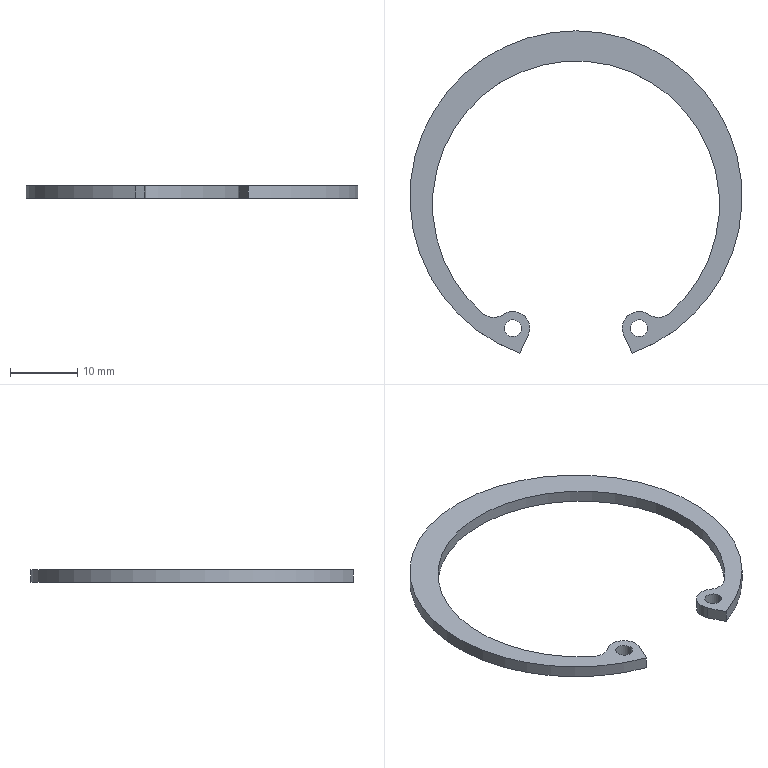Part | STEP file | KS B 1336 - 47x1.8 | 1 solid | 16 faces | box 49.5 x 48.026 x 1.8 mm | volume 847.052 mm3 | cylinder 12 | plane 4 | commonest cylinder face diameters 2.5 x4 5 x4 42.75 x2 49.5 x2
STEP:
#1=CARTESIAN_POINT('',(0.,0.,0.));
#2=DIRECTION('',(0.,0.,1.));
#3=DIRECTION('',(1.,0.,0.));
#4=AXIS2_PLACEMENT_3D('',#1,#2,#3);
#5=CARTESIAN_POINT('',(8.152,-43.058,0.));
#6=VERTEX_POINT('',#5);
#7=CARTESIAN_POINT('',(8.152,-43.058,1.8));
#8=VERTEX_POINT('',#7);
#9=CARTESIAN_POINT('',(8.152,-43.058,0.));
#10=DIRECTION('',(0.,0.,1.));
#11=VECTOR('',#10,1.);
#12=LINE('',#9,#11);
#13=CARTESIAN_POINT('',(9.402,-43.058,0.));
#14=DIRECTION('',(0.,0.,1.));
#15=DIRECTION('',(-1.,0.,0.));
#16=AXIS2_PLACEMENT_3D('',#13,#14,#15);
#17=CYLINDRICAL_SURFACE('',#16,1.25);
#18=CARTESIAN_POINT('',(6.283,0.));
#19=DIRECTION('',(0.,1.));
#20=VECTOR('',#19,1.);
#21=LINE('',#18,#20);
#22=(GEOMETRIC_REPRESENTATION_CONTEXT(2)PARAMETRIC_REPRESENTATION_CONTEXT()REPRESENTATION_CONTEXT('',''));
#23=DEFINITIONAL_REPRESENTATION('',(#21),#22);
#24=PCURVE('',#17,#23);
#25=CARTESIAN_POINT('',(9.402,-43.058,0.));
#26=DIRECTION('',(0.,0.,1.));
#27=DIRECTION('',(-1.,0.,0.));
#28=AXIS2_PLACEMENT_3D('',#25,#26,#27);
#29=CYLINDRICAL_SURFACE('',#28,1.25);
#30=CARTESIAN_POINT('',(0.,0.));
#31=DIRECTION('',(0.,1.));
#32=VECTOR('',#31,1.);
#33=LINE('',#30,#32);
#34=(GEOMETRIC_REPRESENTATION_CONTEXT(2)PARAMETRIC_REPRESENTATION_CONTEXT()REPRESENTATION_CONTEXT('',''));
#35=DEFINITIONAL_REPRESENTATION('',(#33),#34);
#36=PCURVE('',#29,#35);
#37=SURFACE_CURVE('',#12,(#24,#36),.PCURVE_S1.);
#38=EDGE_CURVE('',#6,#8,#37,.T.);
#39=ORIENTED_EDGE('',*,*,#38,.T.);
#40=CARTESIAN_POINT('',(10.652,-43.058,1.8));
#41=VERTEX_POINT('',#40);
#42=CARTESIAN_POINT('',(9.402,-43.058,1.8));
#43=DIRECTION('',(0.,0.,-1.));
#44=DIRECTION('',(-1.,0.,0.));
#45=AXIS2_PLACEMENT_3D('',#42,#43,#44);
#46=CIRCLE('',#45,1.25);
#47=CARTESIAN_POINT('',(6.283,1.8));
#48=DIRECTION('',(-1.,0.));
#49=VECTOR('',#48,1.);
#50=LINE('',#47,#49);
#51=(GEOMETRIC_REPRESENTATION_CONTEXT(2)PARAMETRIC_REPRESENTATION_CONTEXT()REPRESENTATION_CONTEXT('',''));
#52=DEFINITIONAL_REPRESENTATION('',(#50),#51);
#53=PCURVE('',#17,#52);
#54=CARTESIAN_POINT('',(-0.06336,-23.349,1.8));
#55=DIRECTION('',(0.,0.,1.));
#56=DIRECTION('',(1.,0.,0.));
#57=AXIS2_PLACEMENT_3D('',#54,#55,#56);
#58=PLANE('',#57);
#59=CARTESIAN_POINT('',(8.215,-19.708));
#60=CARTESIAN_POINT('',(8.215,-17.543));
#61=CARTESIAN_POINT('',(10.09,-18.626));
#62=CARTESIAN_POINT('',(11.965,-19.708));
#63=CARTESIAN_POINT('',(10.09,-20.791));
#64=CARTESIAN_POINT('',(8.215,-21.873));
#65=CARTESIAN_POINT('',(8.215,-19.708));
#66=(BOUNDED_CURVE()B_SPLINE_CURVE(2,(#59,#60,#61,#62,#63,#64,#65),.UNSPECIFIED.,.T.,.F.)B_SPLINE_CURVE_WITH_KNOTS((1,2,2,2,2,1),(-2.094,0.,2.094,4.189,6.283,8.378),.UNSPECIFIED.)CURVE()GEOMETRIC_REPRESENTATION_ITEM()RATIONAL_B_SPLINE_CURVE((1.,0.5,1.,0.5,1.,0.5,1.))REPRESENTATION_ITEM(''));
#67=(GEOMETRIC_REPRESENTATION_CONTEXT(2)PARAMETRIC_REPRESENTATION_CONTEXT()REPRESENTATION_CONTEXT('',''));
#68=DEFINITIONAL_REPRESENTATION('',(#66),#67);
#69=PCURVE('',#58,#68);
#70=SURFACE_CURVE('',#46,(#53,#69),.PCURVE_S1.);
#71=EDGE_CURVE('',#8,#41,#70,.T.);
#72=ORIENTED_EDGE('',*,*,#71,.T.);
#73=CARTESIAN_POINT('',(10.652,-43.058,0.));
#74=VERTEX_POINT('',#73);
#75=CARTESIAN_POINT('',(10.652,-43.058,0.));
#76=DIRECTION('',(0.,0.,1.));
#77=VECTOR('',#76,1.);
#78=LINE('',#75,#77);
#79=CARTESIAN_POINT('',(3.142,0.));
#80=DIRECTION('',(0.,1.));
#81=VECTOR('',#80,1.);
#82=LINE('',#79,#81);
#83=(GEOMETRIC_REPRESENTATION_CONTEXT(2)PARAMETRIC_REPRESENTATION_CONTEXT()REPRESENTATION_CONTEXT('',''));
#84=DEFINITIONAL_REPRESENTATION('',(#82),#83);
#85=PCURVE('',#17,#84);
#86=CARTESIAN_POINT('',(3.142,0.));
#87=DIRECTION('',(0.,1.));
#88=VECTOR('',#87,1.);
#89=LINE('',#86,#88);
#90=(GEOMETRIC_REPRESENTATION_CONTEXT(2)PARAMETRIC_REPRESENTATION_CONTEXT()REPRESENTATION_CONTEXT('',''));
#91=DEFINITIONAL_REPRESENTATION('',(#89),#90);
#92=PCURVE('',#29,#91);
#93=SURFACE_CURVE('',#78,(#85,#92),.PCURVE_S1.);
#94=EDGE_CURVE('',#74,#41,#93,.T.);
#95=ORIENTED_EDGE('',*,*,#94,.F.);
#96=CARTESIAN_POINT('',(9.402,-43.058,0.));
#97=DIRECTION('',(0.,0.,1.));
#98=DIRECTION('',(-1.,0.,0.));
#99=AXIS2_PLACEMENT_3D('',#96,#97,#98);
#100=CIRCLE('',#99,1.25);
#101=CARTESIAN_POINT('',(0.,0.));
#102=DIRECTION('',(1.,0.));
#103=VECTOR('',#102,1.);
#104=LINE('',#101,#103);
#105=(GEOMETRIC_REPRESENTATION_CONTEXT(2)PARAMETRIC_REPRESENTATION_CONTEXT()REPRESENTATION_CONTEXT('',''));
#106=DEFINITIONAL_REPRESENTATION('',(#104),#105);
#107=PCURVE('',#17,#106);
#108=CARTESIAN_POINT('',(-0.06336,-23.349,0.));
#109=DIRECTION('',(0.,0.,1.));
#110=DIRECTION('',(1.,0.,0.));
#111=AXIS2_PLACEMENT_3D('',#108,#109,#110);
#112=PLANE('',#111);
#113=CARTESIAN_POINT('',(9.465,-19.708));
#114=DIRECTION('',(-1.,0.));
#115=AXIS2_PLACEMENT_2D('',#113,#114);
#116=CIRCLE('',#115,1.25);
#117=(GEOMETRIC_REPRESENTATION_CONTEXT(2)PARAMETRIC_REPRESENTATION_CONTEXT()REPRESENTATION_CONTEXT('',''));
#118=DEFINITIONAL_REPRESENTATION('',(#116),#117);
#119=PCURVE('',#112,#118);
#120=SURFACE_CURVE('',#100,(#107,#119),.PCURVE_S1.);
#121=EDGE_CURVE('',#74,#6,#120,.T.);
#122=ORIENTED_EDGE('',*,*,#121,.T.);
#123=EDGE_LOOP('',(#39,#72,#95,#122));
#124=FACE_BOUND('',#123,.F.);
#125=ADVANCED_FACE('',(#124),#17,.F.);
#126=CARTESIAN_POINT('',(-10.652,-43.058,0.));
#127=VERTEX_POINT('',#126);
#128=CARTESIAN_POINT('',(-10.652,-43.058,1.8));
#129=VERTEX_POINT('',#128);
#130=CARTESIAN_POINT('',(-10.652,-43.058,0.));
#131=DIRECTION('',(0.,0.,1.));
#132=VECTOR('',#131,1.);
#133=LINE('',#130,#132);
#134=CARTESIAN_POINT('',(-9.402,-43.058,0.));
#135=DIRECTION('',(0.,0.,1.));
#136=DIRECTION('',(-1.,0.,0.));
#137=AXIS2_PLACEMENT_3D('',#134,#135,#136);
#138=CYLINDRICAL_SURFACE('',#137,1.25);
#139=CARTESIAN_POINT('',(6.283,0.));
#140=DIRECTION('',(0.,1.));
#141=VECTOR('',#140,1.);
#142=LINE('',#139,#141);
#143=(GEOMETRIC_REPRESENTATION_CONTEXT(2)PARAMETRIC_REPRESENTATION_CONTEXT()REPRESENTATION_CONTEXT('',''));
#144=DEFINITIONAL_REPRESENTATION('',(#142),#143);
#145=PCURVE('',#138,#144);
#146=CARTESIAN_POINT('',(-9.402,-43.058,0.));
#147=DIRECTION('',(0.,0.,1.));
#148=DIRECTION('',(-1.,0.,0.));
#149=AXIS2_PLACEMENT_3D('',#146,#147,#148);
#150=CYLINDRICAL_SURFACE('',#149,1.25);
#151=CARTESIAN_POINT('',(0.,0.));
#152=DIRECTION('',(0.,1.));
#153=VECTOR('',#152,1.);
#154=LINE('',#151,#153);
#155=(GEOMETRIC_REPRESENTATION_CONTEXT(2)PARAMETRIC_REPRESENTATION_CONTEXT()REPRESENTATION_CONTEXT('',''));
#156=DEFINITIONAL_REPRESENTATION('',(#154),#155);
#157=PCURVE('',#150,#156);
#158=SURFACE_CURVE('',#133,(#145,#157),.PCURVE_S1.);
#159=EDGE_CURVE('',#127,#129,#158,.T.);
#160=ORIENTED_EDGE('',*,*,#159,.T.);
#161=CARTESIAN_POINT('',(-8.152,-43.058,1.8));
#162=VERTEX_POINT('',#161);
#163=CARTESIAN_POINT('',(-9.402,-43.058,1.8));
#164=DIRECTION('',(0.,0.,-1.));
#165=DIRECTION('',(-1.,0.,0.));
#166=AXIS2_PLACEMENT_3D('',#163,#164,#165);
#167=CIRCLE('',#166,1.25);
#168=CARTESIAN_POINT('',(6.283,1.8));
#169=DIRECTION('',(-1.,0.));
#170=VECTOR('',#169,1.);
#171=LINE('',#168,#170);
#172=(GEOMETRIC_REPRESENTATION_CONTEXT(2)PARAMETRIC_REPRESENTATION_CONTEXT()REPRESENTATION_CONTEXT('',''));
#173=DEFINITIONAL_REPRESENTATION('',(#171),#172);
#174=PCURVE('',#138,#173);
#175=CARTESIAN_POINT('',(-10.588,-19.708));
#176=CARTESIAN_POINT('',(-10.588,-17.543));
#177=CARTESIAN_POINT('',(-8.713,-18.626));
#178=CARTESIAN_POINT('',(-6.838,-19.708));
#179=CARTESIAN_POINT('',(-8.713,-20.791));
#180=CARTESIAN_POINT('',(-10.588,-21.873));
#181=CARTESIAN_POINT('',(-10.588,-19.708));
#182=(BOUNDED_CURVE()B_SPLINE_CURVE(2,(#175,#176,#177,#178,#179,#180,#181),.UNSPECIFIED.,.T.,.F.)B_SPLINE_CURVE_WITH_KNOTS((1,2,2,2,2,1),(-2.094,0.,2.094,4.189,6.283,8.378),.UNSPECIFIED.)CURVE()GEOMETRIC_REPRESENTATION_ITEM()RATIONAL_B_SPLINE_CURVE((1.,0.5,1.,0.5,1.,0.5,1.))REPRESENTATION_ITEM(''));
#183=(GEOMETRIC_REPRESENTATION_CONTEXT(2)PARAMETRIC_REPRESENTATION_CONTEXT()REPRESENTATION_CONTEXT('',''));
#184=DEFINITIONAL_REPRESENTATION('',(#182),#183);
#185=PCURVE('',#58,#184);
#186=SURFACE_CURVE('',#167,(#174,#185),.PCURVE_S1.);
#187=EDGE_CURVE('',#129,#162,#186,.T.);
#188=ORIENTED_EDGE('',*,*,#187,.T.);
#189=CARTESIAN_POINT('',(-8.152,-43.058,0.));
#190=VERTEX_POINT('',#189);
#191=CARTESIAN_POINT('',(-8.152,-43.058,0.));
#192=DIRECTION('',(0.,0.,1.));
#193=VECTOR('',#192,1.);
#194=LINE('',#191,#193);
#195=CARTESIAN_POINT('',(3.142,0.));
#196=DIRECTION('',(0.,1.));
#197=VECTOR('',#196,1.);
#198=LINE('',#195,#197);
#199=(GEOMETRIC_REPRESENTATION_CONTEXT(2)PARAMETRIC_REPRESENTATION_CONTEXT()REPRESENTATION_CONTEXT('',''));
#200=DEFINITIONAL_REPRESENTATION('',(#198),#199);
#201=PCURVE('',#138,#200);
#202=CARTESIAN_POINT('',(3.142,0.));
#203=DIRECTION('',(0.,1.));
#204=VECTOR('',#203,1.);
#205=LINE('',#202,#204);
#206=(GEOMETRIC_REPRESENTATION_CONTEXT(2)PARAMETRIC_REPRESENTATION_CONTEXT()REPRESENTATION_CONTEXT('',''));
#207=DEFINITIONAL_REPRESENTATION('',(#205),#206);
#208=PCURVE('',#150,#207);
#209=SURFACE_CURVE('',#194,(#201,#208),.PCURVE_S1.);
#210=EDGE_CURVE('',#190,#162,#209,.T.);
#211=ORIENTED_EDGE('',*,*,#210,.F.);
#212=CARTESIAN_POINT('',(-9.402,-43.058,0.));
#213=DIRECTION('',(0.,0.,1.));
#214=DIRECTION('',(-1.,0.,0.));
#215=AXIS2_PLACEMENT_3D('',#212,#213,#214);
#216=CIRCLE('',#215,1.25);
#217=CARTESIAN_POINT('',(0.,0.));
#218=DIRECTION('',(1.,0.));
#219=VECTOR('',#218,1.);
#220=LINE('',#217,#219);
#221=(GEOMETRIC_REPRESENTATION_CONTEXT(2)PARAMETRIC_REPRESENTATION_CONTEXT()REPRESENTATION_CONTEXT('',''));
#222=DEFINITIONAL_REPRESENTATION('',(#220),#221);
#223=PCURVE('',#138,#222);
#224=CARTESIAN_POINT('',(-9.338,-19.708));
#225=DIRECTION('',(-1.,0.));
#226=AXIS2_PLACEMENT_2D('',#224,#225);
#227=CIRCLE('',#226,1.25);
#228=(GEOMETRIC_REPRESENTATION_CONTEXT(2)PARAMETRIC_REPRESENTATION_CONTEXT()REPRESENTATION_CONTEXT('',''));
#229=DEFINITIONAL_REPRESENTATION('',(#227),#228);
#230=PCURVE('',#112,#229);
#231=SURFACE_CURVE('',#216,(#223,#230),.PCURVE_S1.);
#232=EDGE_CURVE('',#190,#127,#231,.T.);
#233=ORIENTED_EDGE('',*,*,#232,.T.);
#234=EDGE_LOOP('',(#160,#188,#211,#233));
#235=FACE_BOUND('',#234,.F.);
#236=ADVANCED_FACE('',(#235),#138,.F.);
#237=CARTESIAN_POINT('',(-13.899,-40.864,0.));
#238=VERTEX_POINT('',#237);
#239=CARTESIAN_POINT('',(-13.899,-40.864,1.8));
#240=VERTEX_POINT('',#239);
#241=CARTESIAN_POINT('',(-13.899,-40.864,0.));
#242=DIRECTION('',(0.,0.,1.));
#243=VECTOR('',#242,1.);
#244=LINE('',#241,#243);
#245=CARTESIAN_POINT('',(0.,-24.625,0.));
#246=DIRECTION('',(0.,0.,1.));
#247=DIRECTION('',(-0.6503,0.7597,0.));
#248=AXIS2_PLACEMENT_3D('',#245,#246,#247);
#249=CYLINDRICAL_SURFACE('',#248,21.375);
#250=CARTESIAN_POINT('',(1.726,0.));
#251=DIRECTION('',(0.,1.));
#252=VECTOR('',#251,1.);
#253=LINE('',#250,#252);
#254=(GEOMETRIC_REPRESENTATION_CONTEXT(2)PARAMETRIC_REPRESENTATION_CONTEXT()REPRESENTATION_CONTEXT('',''));
#255=DEFINITIONAL_REPRESENTATION('',(#253),#254);
#256=PCURVE('',#249,#255);
#257=CARTESIAN_POINT('',(-12.274,-38.965,0.));
#258=DIRECTION('',(0.,0.,1.));
#259=DIRECTION('',(0.6503,0.7597,0.));
#260=AXIS2_PLACEMENT_3D('',#257,#258,#259);
#261=CYLINDRICAL_SURFACE('',#260,2.5);
#262=CARTESIAN_POINT('',(3.142,0.));
#263=DIRECTION('',(0.,1.));
#264=VECTOR('',#263,1.);
#265=LINE('',#262,#264);
#266=(GEOMETRIC_REPRESENTATION_CONTEXT(2)PARAMETRIC_REPRESENTATION_CONTEXT()REPRESENTATION_CONTEXT('',''));
#267=DEFINITIONAL_REPRESENTATION('',(#265),#266);
#268=PCURVE('',#261,#267);
#269=SURFACE_CURVE('',#244,(#256,#268),.PCURVE_S1.);
#270=EDGE_CURVE('',#238,#240,#269,.T.);
#271=ORIENTED_EDGE('',*,*,#270,.T.);
#272=CARTESIAN_POINT('',(-13.899,-8.386,1.8));
#273=VERTEX_POINT('',#272);
#274=CARTESIAN_POINT('',(0.,-24.625,1.8));
#275=DIRECTION('',(0.,0.,1.));
#276=DIRECTION('',(-0.6503,0.7597,0.));
#277=AXIS2_PLACEMENT_3D('',#274,#275,#276);
#278=CIRCLE('',#277,21.375);
#279=CARTESIAN_POINT('',(0.,1.8));
#280=DIRECTION('',(1.,0.));
#281=VECTOR('',#280,1.);
#282=LINE('',#279,#281);
#283=(GEOMETRIC_REPRESENTATION_CONTEXT(2)PARAMETRIC_REPRESENTATION_CONTEXT()REPRESENTATION_CONTEXT('',''));
#284=DEFINITIONAL_REPRESENTATION('',(#282),#283);
#285=PCURVE('',#249,#284);
#286=CARTESIAN_POINT('',(0.06336,-1.276));
#287=DIRECTION('',(-0.6503,0.7597));
#288=AXIS2_PLACEMENT_2D('',#286,#287);
#289=CIRCLE('',#288,21.375);
#290=(GEOMETRIC_REPRESENTATION_CONTEXT(2)PARAMETRIC_REPRESENTATION_CONTEXT()REPRESENTATION_CONTEXT('',''));
#291=DEFINITIONAL_REPRESENTATION('',(#289),#290);
#292=PCURVE('',#58,#291);
#293=SURFACE_CURVE('',#278,(#285,#292),.PCURVE_S1.);
#294=EDGE_CURVE('',#273,#240,#293,.T.);
#295=ORIENTED_EDGE('',*,*,#294,.F.);
#296=CARTESIAN_POINT('',(-13.899,-8.386,0.));
#297=VERTEX_POINT('',#296);
#298=CARTESIAN_POINT('',(-13.899,-8.386,0.));
#299=DIRECTION('',(0.,0.,1.));
#300=VECTOR('',#299,1.);
#301=LINE('',#298,#300);
#302=CARTESIAN_POINT('',(0.,0.));
#303=DIRECTION('',(0.,1.));
#304=VECTOR('',#303,1.);
#305=LINE('',#302,#304);
#306=(GEOMETRIC_REPRESENTATION_CONTEXT(2)PARAMETRIC_REPRESENTATION_CONTEXT()REPRESENTATION_CONTEXT('',''));
#307=DEFINITIONAL_REPRESENTATION('',(#305),#306);
#308=PCURVE('',#249,#307);
#309=CARTESIAN_POINT('',(0.,-24.625,0.));
#310=DIRECTION('',(0.,0.,1.));
#311=DIRECTION('',(-0.6503,0.7597,0.));
#312=AXIS2_PLACEMENT_3D('',#309,#310,#311);
#313=CYLINDRICAL_SURFACE('',#312,21.375);
#314=CARTESIAN_POINT('',(6.283,0.));
#315=DIRECTION('',(0.,1.));
#316=VECTOR('',#315,1.);
#317=LINE('',#314,#316);
#318=(GEOMETRIC_REPRESENTATION_CONTEXT(2)PARAMETRIC_REPRESENTATION_CONTEXT()REPRESENTATION_CONTEXT('',''));
#319=DEFINITIONAL_REPRESENTATION('',(#317),#318);
#320=PCURVE('',#313,#319);
#321=SURFACE_CURVE('',#301,(#308,#320),.PCURVE_S1.);
#322=EDGE_CURVE('',#297,#273,#321,.T.);
#323=ORIENTED_EDGE('',*,*,#322,.F.);
#324=CARTESIAN_POINT('',(0.,-24.625,0.));
#325=DIRECTION('',(0.,0.,-1.));
#326=DIRECTION('',(-0.6503,0.7597,0.));
#327=AXIS2_PLACEMENT_3D('',#324,#325,#326);
#328=CIRCLE('',#327,21.375);
#329=CARTESIAN_POINT('',(6.283,0.));
#330=DIRECTION('',(-1.,0.));
#331=VECTOR('',#330,1.);
#332=LINE('',#329,#331);
#333=(GEOMETRIC_REPRESENTATION_CONTEXT(2)PARAMETRIC_REPRESENTATION_CONTEXT()REPRESENTATION_CONTEXT('',''));
#334=DEFINITIONAL_REPRESENTATION('',(#332),#333);
#335=PCURVE('',#249,#334);
#336=CARTESIAN_POINT('',(-13.836,14.963));
#337=CARTESIAN_POINT('',(14.291,39.037));
#338=CARTESIAN_POINT('',(21.076,2.642));
#339=CARTESIAN_POINT('',(27.862,-33.754));
#340=CARTESIAN_POINT('',(-7.05,-21.432));
#341=CARTESIAN_POINT('',(-41.963,-9.111));
#342=CARTESIAN_POINT('',(-13.836,14.963));
#343=(BOUNDED_CURVE()B_SPLINE_CURVE(2,(#336,#337,#338,#339,#340,#341,#342),.UNSPECIFIED.,.T.,.F.)B_SPLINE_CURVE_WITH_KNOTS((1,2,2,2,2,1),(-2.094,0.,2.094,4.189,6.283,8.378),.UNSPECIFIED.)CURVE()GEOMETRIC_REPRESENTATION_ITEM()RATIONAL_B_SPLINE_CURVE((1.,0.5,1.,0.5,1.,0.5,1.))REPRESENTATION_ITEM(''));
#344=(GEOMETRIC_REPRESENTATION_CONTEXT(2)PARAMETRIC_REPRESENTATION_CONTEXT()REPRESENTATION_CONTEXT('',''));
#345=DEFINITIONAL_REPRESENTATION('',(#343),#344);
#346=PCURVE('',#112,#345);
#347=SURFACE_CURVE('',#328,(#335,#346),.PCURVE_S1.);
#348=EDGE_CURVE('',#238,#297,#347,.T.);
#349=ORIENTED_EDGE('',*,*,#348,.F.);
#350=EDGE_LOOP('',(#271,#295,#323,#349));
#351=FACE_BOUND('',#350,.F.);
#352=ADVANCED_FACE('',(#351),#249,.F.);
#353=CARTESIAN_POINT('',(8.415,-46.776,0.));
#354=VERTEX_POINT('',#353);
#355=CARTESIAN_POINT('',(0.,1.25,0.));
#356=VERTEX_POINT('',#355);
#357=CARTESIAN_POINT('',(0.,-23.5,0.));
#358=DIRECTION('',(0.,0.,1.));
#359=DIRECTION('',(0.34,-0.9404,0.));
#360=AXIS2_PLACEMENT_3D('',#357,#358,#359);
#361=CIRCLE('',#360,24.75);
#362=CARTESIAN_POINT('',(0.,-23.5,0.));
#363=DIRECTION('',(0.,0.,1.));
#364=DIRECTION('',(0.,1.,0.));
#365=AXIS2_PLACEMENT_3D('',#362,#363,#364);
#366=CYLINDRICAL_SURFACE('',#365,24.75);
#367=CARTESIAN_POINT('',(3.489,0.));
#368=DIRECTION('',(1.,0.));
#369=VECTOR('',#368,1.);
#370=LINE('',#367,#369);
#371=(GEOMETRIC_REPRESENTATION_CONTEXT(2)PARAMETRIC_REPRESENTATION_CONTEXT()REPRESENTATION_CONTEXT('',''));
#372=DEFINITIONAL_REPRESENTATION('',(#370),#371);
#373=PCURVE('',#366,#372);
#374=CARTESIAN_POINT('',(0.06336,-0.1508));
#375=DIRECTION('',(0.34,-0.9404));
#376=AXIS2_PLACEMENT_2D('',#374,#375);
#377=CIRCLE('',#376,24.75);
#378=(GEOMETRIC_REPRESENTATION_CONTEXT(2)PARAMETRIC_REPRESENTATION_CONTEXT()REPRESENTATION_CONTEXT('',''));
#379=DEFINITIONAL_REPRESENTATION('',(#377),#378);
#380=PCURVE('',#112,#379);
#381=SURFACE_CURVE('',#361,(#373,#380),.PCURVE_S1.);
#382=EDGE_CURVE('',#354,#356,#381,.T.);
#383=ORIENTED_EDGE('',*,*,#382,.T.);
#384=CARTESIAN_POINT('',(0.,1.25,1.8));
#385=VERTEX_POINT('',#384);
#386=CARTESIAN_POINT('',(0.,1.25,0.));
#387=DIRECTION('',(0.,0.,1.));
#388=VECTOR('',#387,1.);
#389=LINE('',#386,#388);
#390=CARTESIAN_POINT('',(6.283,0.));
#391=DIRECTION('',(0.,1.));
#392=VECTOR('',#391,1.);
#393=LINE('',#390,#392);
#394=(GEOMETRIC_REPRESENTATION_CONTEXT(2)PARAMETRIC_REPRESENTATION_CONTEXT()REPRESENTATION_CONTEXT('',''));
#395=DEFINITIONAL_REPRESENTATION('',(#393),#394);
#396=PCURVE('',#366,#395);
#397=CARTESIAN_POINT('',(0.,-23.5,0.));
#398=DIRECTION('',(0.,0.,1.));
#399=DIRECTION('',(0.,1.,0.));
#400=AXIS2_PLACEMENT_3D('',#397,#398,#399);
#401=CYLINDRICAL_SURFACE('',#400,24.75);
#402=CARTESIAN_POINT('',(0.,0.));
#403=DIRECTION('',(0.,1.));
#404=VECTOR('',#403,1.);
#405=LINE('',#402,#404);
#406=(GEOMETRIC_REPRESENTATION_CONTEXT(2)PARAMETRIC_REPRESENTATION_CONTEXT()REPRESENTATION_CONTEXT('',''));
#407=DEFINITIONAL_REPRESENTATION('',(#405),#406);
#408=PCURVE('',#401,#407);
#409=SURFACE_CURVE('',#389,(#396,#408),.PCURVE_S1.);
#410=EDGE_CURVE('',#356,#385,#409,.T.);
#411=ORIENTED_EDGE('',*,*,#410,.T.);
#412=CARTESIAN_POINT('',(8.415,-46.776,1.8));
#413=VERTEX_POINT('',#412);
#414=CARTESIAN_POINT('',(0.,-23.5,1.8));
#415=DIRECTION('',(0.,0.,-1.));
#416=DIRECTION('',(0.34,-0.9404,0.));
#417=AXIS2_PLACEMENT_3D('',#414,#415,#416);
#418=CIRCLE('',#417,24.75);
#419=CARTESIAN_POINT('',(9.772,1.8));
#420=DIRECTION('',(-1.,0.));
#421=VECTOR('',#420,1.);
#422=LINE('',#419,#421);
#423=(GEOMETRIC_REPRESENTATION_CONTEXT(2)PARAMETRIC_REPRESENTATION_CONTEXT()REPRESENTATION_CONTEXT('',''));
#424=DEFINITIONAL_REPRESENTATION('',(#422),#423);
#425=PCURVE('',#366,#424);
#426=CARTESIAN_POINT('',(8.478,-23.426));
#427=CARTESIAN_POINT('',(-31.836,-38.002));
#428=CARTESIAN_POINT('',(-24.301,4.199));
#429=CARTESIAN_POINT('',(-16.767,46.4));
#430=CARTESIAN_POINT('',(16.013,18.775));
#431=CARTESIAN_POINT('',(48.793,-8.851));
#432=CARTESIAN_POINT('',(8.478,-23.426));
#433=(BOUNDED_CURVE()B_SPLINE_CURVE(2,(#426,#427,#428,#429,#430,#431,#432),.UNSPECIFIED.,.T.,.F.)B_SPLINE_CURVE_WITH_KNOTS((1,2,2,2,2,1),(-2.094,0.,2.094,4.189,6.283,8.378),.UNSPECIFIED.)CURVE()GEOMETRIC_REPRESENTATION_ITEM()RATIONAL_B_SPLINE_CURVE((1.,0.5,1.,0.5,1.,0.5,1.))REPRESENTATION_ITEM(''));
#434=(GEOMETRIC_REPRESENTATION_CONTEXT(2)PARAMETRIC_REPRESENTATION_CONTEXT()REPRESENTATION_CONTEXT('',''));
#435=DEFINITIONAL_REPRESENTATION('',(#433),#434);
#436=PCURVE('',#58,#435);
#437=SURFACE_CURVE('',#418,(#425,#436),.PCURVE_S1.);
#438=EDGE_CURVE('',#385,#413,#437,.T.);
#439=ORIENTED_EDGE('',*,*,#438,.T.);
#440=CARTESIAN_POINT('',(8.415,-46.776,0.));
#441=DIRECTION('',(0.,0.,1.));
#442=VECTOR('',#441,1.);
#443=LINE('',#440,#442);
#444=CARTESIAN_POINT('',(3.489,0.));
#445=DIRECTION('',(0.,1.));
#446=VECTOR('',#445,1.);
#447=LINE('',#444,#446);
#448=(GEOMETRIC_REPRESENTATION_CONTEXT(2)PARAMETRIC_REPRESENTATION_CONTEXT()REPRESENTATION_CONTEXT('',''));
#449=DEFINITIONAL_REPRESENTATION('',(#447),#448);
#450=PCURVE('',#366,#449);
#451=CARTESIAN_POINT('',(8.415,-46.776,0.));
#452=DIRECTION('',(-0.9013,-0.4333,0.));
#453=DIRECTION('',(-0.4333,0.9013,0.));
#454=AXIS2_PLACEMENT_3D('',#451,#452,#453);
#455=PLANE('',#454);
#456=CARTESIAN_POINT('',(0.,0.));
#457=DIRECTION('',(0.,-1.));
#458=VECTOR('',#457,1.);
#459=LINE('',#456,#458);
#460=(GEOMETRIC_REPRESENTATION_CONTEXT(2)PARAMETRIC_REPRESENTATION_CONTEXT()REPRESENTATION_CONTEXT('',''));
#461=DEFINITIONAL_REPRESENTATION('',(#459),#460);
#462=PCURVE('',#455,#461);
#463=SURFACE_CURVE('',#443,(#450,#462),.PCURVE_S1.);
#464=EDGE_CURVE('',#354,#413,#463,.T.);
#465=ORIENTED_EDGE('',*,*,#464,.F.);
#466=EDGE_LOOP('',(#383,#411,#439,#465));
#467=FACE_BOUND('',#466,.T.);
#468=ADVANCED_FACE('',(#467),#366,.T.);
#469=ORIENTED_EDGE('',*,*,#187,.T.);
#470=CARTESIAN_POINT('',(-9.402,-43.058,1.8));
#471=DIRECTION('',(0.,0.,-1.));
#472=DIRECTION('',(-1.,0.,0.));
#473=AXIS2_PLACEMENT_3D('',#470,#471,#472);
#474=CIRCLE('',#473,1.25);
#475=CARTESIAN_POINT('',(-10.588,-19.708));
#476=CARTESIAN_POINT('',(-10.588,-17.543));
#477=CARTESIAN_POINT('',(-8.713,-18.626));
#478=CARTESIAN_POINT('',(-6.838,-19.708));
#479=CARTESIAN_POINT('',(-8.713,-20.791));
#480=CARTESIAN_POINT('',(-10.588,-21.873));
#481=CARTESIAN_POINT('',(-10.588,-19.708));
#482=(BOUNDED_CURVE()B_SPLINE_CURVE(2,(#475,#476,#477,#478,#479,#480,#481),.UNSPECIFIED.,.T.,.F.)B_SPLINE_CURVE_WITH_KNOTS((1,2,2,2,2,1),(-2.094,0.,2.094,4.189,6.283,8.378),.UNSPECIFIED.)CURVE()GEOMETRIC_REPRESENTATION_ITEM()RATIONAL_B_SPLINE_CURVE((1.,0.5,1.,0.5,1.,0.5,1.))REPRESENTATION_ITEM(''));
#483=(GEOMETRIC_REPRESENTATION_CONTEXT(2)PARAMETRIC_REPRESENTATION_CONTEXT()REPRESENTATION_CONTEXT('',''));
#484=DEFINITIONAL_REPRESENTATION('',(#482),#483);
#485=PCURVE('',#58,#484);
#486=CARTESIAN_POINT('',(6.283,1.8));
#487=DIRECTION('',(-1.,0.));
#488=VECTOR('',#487,1.);
#489=LINE('',#486,#488);
#490=(GEOMETRIC_REPRESENTATION_CONTEXT(2)PARAMETRIC_REPRESENTATION_CONTEXT()REPRESENTATION_CONTEXT('',''));
#491=DEFINITIONAL_REPRESENTATION('',(#489),#490);
#492=PCURVE('',#150,#491);
#493=SURFACE_CURVE('',#474,(#485,#492),.PCURVE_S1.);
#494=EDGE_CURVE('',#162,#129,#493,.T.);
#495=ORIENTED_EDGE('',*,*,#494,.T.);
#496=EDGE_LOOP('',(#469,#495));
#497=FACE_BOUND('',#496,.T.);
#498=ORIENTED_EDGE('',*,*,#71,.T.);
#499=CARTESIAN_POINT('',(9.402,-43.058,1.8));
#500=DIRECTION('',(0.,0.,-1.));
#501=DIRECTION('',(-1.,0.,0.));
#502=AXIS2_PLACEMENT_3D('',#499,#500,#501);
#503=CIRCLE('',#502,1.25);
#504=CARTESIAN_POINT('',(8.215,-19.708));
#505=CARTESIAN_POINT('',(8.215,-17.543));
#506=CARTESIAN_POINT('',(10.09,-18.626));
#507=CARTESIAN_POINT('',(11.965,-19.708));
#508=CARTESIAN_POINT('',(10.09,-20.791));
#509=CARTESIAN_POINT('',(8.215,-21.873));
#510=CARTESIAN_POINT('',(8.215,-19.708));
#511=(BOUNDED_CURVE()B_SPLINE_CURVE(2,(#504,#505,#506,#507,#508,#509,#510),.UNSPECIFIED.,.T.,.F.)B_SPLINE_CURVE_WITH_KNOTS((1,2,2,2,2,1),(-2.094,0.,2.094,4.189,6.283,8.378),.UNSPECIFIED.)CURVE()GEOMETRIC_REPRESENTATION_ITEM()RATIONAL_B_SPLINE_CURVE((1.,0.5,1.,0.5,1.,0.5,1.))REPRESENTATION_ITEM(''));
#512=(GEOMETRIC_REPRESENTATION_CONTEXT(2)PARAMETRIC_REPRESENTATION_CONTEXT()REPRESENTATION_CONTEXT('',''));
#513=DEFINITIONAL_REPRESENTATION('',(#511),#512);
#514=PCURVE('',#58,#513);
#515=CARTESIAN_POINT('',(6.283,1.8));
#516=DIRECTION('',(-1.,0.));
#517=VECTOR('',#516,1.);
#518=LINE('',#515,#517);
#519=(GEOMETRIC_REPRESENTATION_CONTEXT(2)PARAMETRIC_REPRESENTATION_CONTEXT()REPRESENTATION_CONTEXT('',''));
#520=DEFINITIONAL_REPRESENTATION('',(#518),#519);
#521=PCURVE('',#29,#520);
#522=SURFACE_CURVE('',#503,(#514,#521),.PCURVE_S1.);
#523=EDGE_CURVE('',#41,#8,#522,.T.);
#524=ORIENTED_EDGE('',*,*,#523,.T.);
#525=EDGE_LOOP('',(#498,#524));
#526=FACE_BOUND('',#525,.T.);
#527=CARTESIAN_POINT('',(13.899,-40.864,1.8));
#528=VERTEX_POINT('',#527);
#529=CARTESIAN_POINT('',(0.,-24.625,1.8));
#530=DIRECTION('',(0.,0.,1.));
#531=DIRECTION('',(-0.6503,0.7597,0.));
#532=AXIS2_PLACEMENT_3D('',#529,#530,#531);
#533=CIRCLE('',#532,21.375);
#534=CARTESIAN_POINT('',(0.06336,-1.276));
#535=DIRECTION('',(-0.6503,0.7597));
#536=AXIS2_PLACEMENT_2D('',#534,#535);
#537=CIRCLE('',#536,21.375);
#538=(GEOMETRIC_REPRESENTATION_CONTEXT(2)PARAMETRIC_REPRESENTATION_CONTEXT()REPRESENTATION_CONTEXT('',''));
#539=DEFINITIONAL_REPRESENTATION('',(#537),#538);
#540=PCURVE('',#58,#539);
#541=CARTESIAN_POINT('',(0.,1.8));
#542=DIRECTION('',(1.,0.));
#543=VECTOR('',#542,1.);
#544=LINE('',#541,#543);
#545=(GEOMETRIC_REPRESENTATION_CONTEXT(2)PARAMETRIC_REPRESENTATION_CONTEXT()REPRESENTATION_CONTEXT('',''));
#546=DEFINITIONAL_REPRESENTATION('',(#544),#545);
#547=PCURVE('',#313,#546);
#548=SURFACE_CURVE('',#533,(#540,#547),.PCURVE_S1.);
#549=EDGE_CURVE('',#528,#273,#548,.T.);
#550=ORIENTED_EDGE('',*,*,#549,.F.);
#551=CARTESIAN_POINT('',(10.838,-41.011,1.8));
#552=VERTEX_POINT('',#551);
#553=CARTESIAN_POINT('',(12.274,-38.965,1.8));
#554=DIRECTION('',(0.,0.,1.));
#555=DIRECTION('',(0.5744,0.8186,0.));
#556=AXIS2_PLACEMENT_3D('',#553,#554,#555);
#557=CIRCLE('',#556,2.5);
#558=CARTESIAN_POINT('',(12.337,-15.615));
#559=DIRECTION('',(0.5744,0.8186));
#560=AXIS2_PLACEMENT_2D('',#558,#559);
#561=CIRCLE('',#560,2.5);
#562=(GEOMETRIC_REPRESENTATION_CONTEXT(2)PARAMETRIC_REPRESENTATION_CONTEXT()REPRESENTATION_CONTEXT('',''));
#563=DEFINITIONAL_REPRESENTATION('',(#561),#562);
#564=PCURVE('',#58,#563);
#565=CARTESIAN_POINT('',(12.274,-38.965,0.));
#566=DIRECTION('',(0.,0.,1.));
#567=DIRECTION('',(0.5744,0.8186,0.));
#568=AXIS2_PLACEMENT_3D('',#565,#566,#567);
#569=CYLINDRICAL_SURFACE('',#568,2.5);
#570=CARTESIAN_POINT('',(0.,1.8));
#571=DIRECTION('',(1.,0.));
#572=VECTOR('',#571,1.);
#573=LINE('',#570,#572);
#574=(GEOMETRIC_REPRESENTATION_CONTEXT(2)PARAMETRIC_REPRESENTATION_CONTEXT()REPRESENTATION_CONTEXT('',''));
#575=DEFINITIONAL_REPRESENTATION('',(#573),#574);
#576=PCURVE('',#569,#575);
#577=SURFACE_CURVE('',#557,(#564,#576),.PCURVE_S1.);
#578=EDGE_CURVE('',#552,#528,#577,.T.);
#579=ORIENTED_EDGE('',*,*,#578,.F.);
#580=CARTESIAN_POINT('',(7.148,-44.141,1.8));
#581=VERTEX_POINT('',#580);
#582=CARTESIAN_POINT('',(9.402,-43.058,1.8));
#583=DIRECTION('',(0.,0.,-1.));
#584=DIRECTION('',(0.5744,0.8186,0.));
#585=AXIS2_PLACEMENT_3D('',#582,#583,#584);
#586=CIRCLE('',#585,2.5);
#587=CARTESIAN_POINT('',(10.901,-17.662));
#588=CARTESIAN_POINT('',(14.446,-20.149));
#589=CARTESIAN_POINT('',(10.519,-21.975));
#590=CARTESIAN_POINT('',(6.593,-23.801));
#591=CARTESIAN_POINT('',(6.975,-19.488));
#592=CARTESIAN_POINT('',(7.356,-15.175));
#593=CARTESIAN_POINT('',(10.901,-17.662));
#594=(BOUNDED_CURVE()B_SPLINE_CURVE(2,(#587,#588,#589,#590,#591,#592,#593),.UNSPECIFIED.,.T.,.F.)B_SPLINE_CURVE_WITH_KNOTS((1,2,2,2,2,1),(-2.094,0.,2.094,4.189,6.283,8.378),.UNSPECIFIED.)CURVE()GEOMETRIC_REPRESENTATION_ITEM()RATIONAL_B_SPLINE_CURVE((1.,0.5,1.,0.5,1.,0.5,1.))REPRESENTATION_ITEM(''));
#595=(GEOMETRIC_REPRESENTATION_CONTEXT(2)PARAMETRIC_REPRESENTATION_CONTEXT()REPRESENTATION_CONTEXT('',''));
#596=DEFINITIONAL_REPRESENTATION('',(#594),#595);
#597=PCURVE('',#58,#596);
#598=CARTESIAN_POINT('',(9.402,-43.058,0.));
#599=DIRECTION('',(0.,0.,1.));
#600=DIRECTION('',(0.5744,0.8186,0.));
#601=AXIS2_PLACEMENT_3D('',#598,#599,#600);
#602=CYLINDRICAL_SURFACE('',#601,2.5);
#603=CARTESIAN_POINT('',(6.283,1.8));
#604=DIRECTION('',(-1.,0.));
#605=VECTOR('',#604,1.);
#606=LINE('',#603,#605);
#607=(GEOMETRIC_REPRESENTATION_CONTEXT(2)PARAMETRIC_REPRESENTATION_CONTEXT()REPRESENTATION_CONTEXT('',''));
#608=DEFINITIONAL_REPRESENTATION('',(#606),#607);
#609=PCURVE('',#602,#608);
#610=SURFACE_CURVE('',#586,(#597,#609),.PCURVE_S1.);
#611=EDGE_CURVE('',#581,#552,#610,.T.);
#612=ORIENTED_EDGE('',*,*,#611,.F.);
#613=CARTESIAN_POINT('',(7.148,-44.141,1.8));
#614=DIRECTION('',(-0.4333,0.9013,0.));
#615=VECTOR('',#614,1.);
#616=LINE('',#613,#615);
#617=CARTESIAN_POINT('',(7.212,-20.792));
#618=DIRECTION('',(-0.4333,0.9013));
#619=VECTOR('',#618,1.);
#620=LINE('',#617,#619);
#621=(GEOMETRIC_REPRESENTATION_CONTEXT(2)PARAMETRIC_REPRESENTATION_CONTEXT()REPRESENTATION_CONTEXT('',''));
#622=DEFINITIONAL_REPRESENTATION('',(#620),#621);
#623=PCURVE('',#58,#622);
#624=CARTESIAN_POINT('',(2.923,-1.8));
#625=DIRECTION('',(1.,0.));
#626=VECTOR('',#625,1.);
#627=LINE('',#624,#626);
#628=(GEOMETRIC_REPRESENTATION_CONTEXT(2)PARAMETRIC_REPRESENTATION_CONTEXT()REPRESENTATION_CONTEXT('',''));
#629=DEFINITIONAL_REPRESENTATION('',(#627),#628);
#630=PCURVE('',#455,#629);
#631=SURFACE_CURVE('',#616,(#623,#630),.PCURVE_S1.);
#632=EDGE_CURVE('',#413,#581,#631,.T.);
#633=ORIENTED_EDGE('',*,*,#632,.F.);
#634=ORIENTED_EDGE('',*,*,#438,.F.);
#635=CARTESIAN_POINT('',(-8.415,-46.776,1.8));
#636=VERTEX_POINT('',#635);
#637=CARTESIAN_POINT('',(0.,-23.5,1.8));
#638=DIRECTION('',(0.,0.,-1.));
#639=DIRECTION('',(0.34,-0.9404,0.));
#640=AXIS2_PLACEMENT_3D('',#637,#638,#639);
#641=CIRCLE('',#640,24.75);
#642=CARTESIAN_POINT('',(8.478,-23.426));
#643=CARTESIAN_POINT('',(-31.836,-38.002));
#644=CARTESIAN_POINT('',(-24.301,4.199));
#645=CARTESIAN_POINT('',(-16.767,46.4));
#646=CARTESIAN_POINT('',(16.013,18.775));
#647=CARTESIAN_POINT('',(48.793,-8.851));
#648=CARTESIAN_POINT('',(8.478,-23.426));
#649=(BOUNDED_CURVE()B_SPLINE_CURVE(2,(#642,#643,#644,#645,#646,#647,#648),.UNSPECIFIED.,.T.,.F.)B_SPLINE_CURVE_WITH_KNOTS((1,2,2,2,2,1),(-2.094,0.,2.094,4.189,6.283,8.378),.UNSPECIFIED.)CURVE()GEOMETRIC_REPRESENTATION_ITEM()RATIONAL_B_SPLINE_CURVE((1.,0.5,1.,0.5,1.,0.5,1.))REPRESENTATION_ITEM(''));
#650=(GEOMETRIC_REPRESENTATION_CONTEXT(2)PARAMETRIC_REPRESENTATION_CONTEXT()REPRESENTATION_CONTEXT('',''));
#651=DEFINITIONAL_REPRESENTATION('',(#649),#650);
#652=PCURVE('',#58,#651);
#653=CARTESIAN_POINT('',(3.489,1.8));
#654=DIRECTION('',(-1.,0.));
#655=VECTOR('',#654,1.);
#656=LINE('',#653,#655);
#657=(GEOMETRIC_REPRESENTATION_CONTEXT(2)PARAMETRIC_REPRESENTATION_CONTEXT()REPRESENTATION_CONTEXT('',''));
#658=DEFINITIONAL_REPRESENTATION('',(#656),#657);
#659=PCURVE('',#401,#658);
#660=SURFACE_CURVE('',#641,(#652,#659),.PCURVE_S1.);
#661=EDGE_CURVE('',#636,#385,#660,.T.);
#662=ORIENTED_EDGE('',*,*,#661,.F.);
#663=CARTESIAN_POINT('',(-7.148,-44.141,1.8));
#664=VERTEX_POINT('',#663);
#665=CARTESIAN_POINT('',(-8.415,-46.776,1.8));
#666=DIRECTION('',(-0.4333,-0.9013,0.));
#667=VECTOR('',#666,1.);
#668=LINE('',#665,#667);
#669=CARTESIAN_POINT('',(-8.352,-23.426));
#670=DIRECTION('',(-0.4333,-0.9013));
#671=VECTOR('',#670,1.);
#672=LINE('',#669,#671);
#673=(GEOMETRIC_REPRESENTATION_CONTEXT(2)PARAMETRIC_REPRESENTATION_CONTEXT()REPRESENTATION_CONTEXT('',''));
#674=DEFINITIONAL_REPRESENTATION('',(#672),#673);
#675=PCURVE('',#58,#674);
#676=CARTESIAN_POINT('',(-7.148,-44.141,0.));
#677=DIRECTION('',(0.9013,-0.4333,0.));
#678=DIRECTION('',(0.,0.,-1.));
#679=AXIS2_PLACEMENT_3D('',#676,#677,#678);
#680=PLANE('',#679);
#681=CARTESIAN_POINT('',(-1.8,-2.923));
#682=DIRECTION('',(0.,-1.));
#683=VECTOR('',#682,1.);
#684=LINE('',#681,#683);
#685=(GEOMETRIC_REPRESENTATION_CONTEXT(2)PARAMETRIC_REPRESENTATION_CONTEXT()REPRESENTATION_CONTEXT('',''));
#686=DEFINITIONAL_REPRESENTATION('',(#684),#685);
#687=PCURVE('',#680,#686);
#688=SURFACE_CURVE('',#668,(#675,#687),.PCURVE_S1.);
#689=EDGE_CURVE('',#664,#636,#688,.T.);
#690=ORIENTED_EDGE('',*,*,#689,.F.);
#691=CARTESIAN_POINT('',(-10.838,-41.011,1.8));
#692=VERTEX_POINT('',#691);
#693=CARTESIAN_POINT('',(-9.402,-43.058,1.8));
#694=DIRECTION('',(0.,0.,-1.));
#695=DIRECTION('',(0.9013,-0.4333,0.));
#696=AXIS2_PLACEMENT_3D('',#693,#694,#695);
#697=CIRCLE('',#696,2.5);
#698=CARTESIAN_POINT('',(-7.085,-20.792));
#699=CARTESIAN_POINT('',(-8.961,-24.694));
#700=CARTESIAN_POINT('',(-11.403,-21.118));
#701=CARTESIAN_POINT('',(-13.845,-17.542));
#702=CARTESIAN_POINT('',(-9.527,-17.216));
#703=CARTESIAN_POINT('',(-5.209,-16.889));
#704=CARTESIAN_POINT('',(-7.085,-20.792));
#705=(BOUNDED_CURVE()B_SPLINE_CURVE(2,(#698,#699,#700,#701,#702,#703,#704),.UNSPECIFIED.,.T.,.F.)B_SPLINE_CURVE_WITH_KNOTS((1,2,2,2,2,1),(-2.094,0.,2.094,4.189,6.283,8.378),.UNSPECIFIED.)CURVE()GEOMETRIC_REPRESENTATION_ITEM()RATIONAL_B_SPLINE_CURVE((1.,0.5,1.,0.5,1.,0.5,1.))REPRESENTATION_ITEM(''));
#706=(GEOMETRIC_REPRESENTATION_CONTEXT(2)PARAMETRIC_REPRESENTATION_CONTEXT()REPRESENTATION_CONTEXT('',''));
#707=DEFINITIONAL_REPRESENTATION('',(#705),#706);
#708=PCURVE('',#58,#707);
#709=CARTESIAN_POINT('',(-9.402,-43.058,0.));
#710=DIRECTION('',(0.,0.,1.));
#711=DIRECTION('',(0.9013,-0.4333,0.));
#712=AXIS2_PLACEMENT_3D('',#709,#710,#711);
#713=CYLINDRICAL_SURFACE('',#712,2.5);
#714=CARTESIAN_POINT('',(6.283,1.8));
#715=DIRECTION('',(-1.,0.));
#716=VECTOR('',#715,1.);
#717=LINE('',#714,#716);
#718=(GEOMETRIC_REPRESENTATION_CONTEXT(2)PARAMETRIC_REPRESENTATION_CONTEXT()REPRESENTATION_CONTEXT('',''));
#719=DEFINITIONAL_REPRESENTATION('',(#717),#718);
#720=PCURVE('',#713,#719);
#721=SURFACE_CURVE('',#697,(#708,#720),.PCURVE_S1.);
#722=EDGE_CURVE('',#692,#664,#721,.T.);
#723=ORIENTED_EDGE('',*,*,#722,.F.);
#724=CARTESIAN_POINT('',(-12.274,-38.965,1.8));
#725=DIRECTION('',(0.,0.,1.));
#726=DIRECTION('',(0.6503,0.7597,0.));
#727=AXIS2_PLACEMENT_3D('',#724,#725,#726);
#728=CIRCLE('',#727,2.5);
#729=CARTESIAN_POINT('',(-12.21,-15.615));
#730=DIRECTION('',(0.6503,0.7597));
#731=AXIS2_PLACEMENT_2D('',#729,#730);
#732=CIRCLE('',#731,2.5);
#733=(GEOMETRIC_REPRESENTATION_CONTEXT(2)PARAMETRIC_REPRESENTATION_CONTEXT()REPRESENTATION_CONTEXT('',''));
#734=DEFINITIONAL_REPRESENTATION('',(#732),#733);
#735=PCURVE('',#58,#734);
#736=CARTESIAN_POINT('',(0.,1.8));
#737=DIRECTION('',(1.,0.));
#738=VECTOR('',#737,1.);
#739=LINE('',#736,#738);
#740=(GEOMETRIC_REPRESENTATION_CONTEXT(2)PARAMETRIC_REPRESENTATION_CONTEXT()REPRESENTATION_CONTEXT('',''));
#741=DEFINITIONAL_REPRESENTATION('',(#739),#740);
#742=PCURVE('',#261,#741);
#743=SURFACE_CURVE('',#728,(#735,#742),.PCURVE_S1.);
#744=EDGE_CURVE('',#240,#692,#743,.T.);
#745=ORIENTED_EDGE('',*,*,#744,.F.);
#746=ORIENTED_EDGE('',*,*,#294,.F.);
#747=EDGE_LOOP('',(#550,#579,#612,#633,#634,#662,#690,#723,#745,#746));
#748=FACE_BOUND('',#747,.T.);
#749=ADVANCED_FACE('',(#497,#526,#748),#58,.T.);
#750=CARTESIAN_POINT('',(-9.402,-43.058,0.));
#751=DIRECTION('',(0.,0.,1.));
#752=DIRECTION('',(-1.,0.,0.));
#753=AXIS2_PLACEMENT_3D('',#750,#751,#752);
#754=CIRCLE('',#753,1.25);
#755=CARTESIAN_POINT('',(-9.338,-19.708));
#756=DIRECTION('',(-1.,0.));
#757=AXIS2_PLACEMENT_2D('',#755,#756);
#758=CIRCLE('',#757,1.25);
#759=(GEOMETRIC_REPRESENTATION_CONTEXT(2)PARAMETRIC_REPRESENTATION_CONTEXT()REPRESENTATION_CONTEXT('',''));
#760=DEFINITIONAL_REPRESENTATION('',(#758),#759);
#761=PCURVE('',#112,#760);
#762=CARTESIAN_POINT('',(0.,0.));
#763=DIRECTION('',(1.,0.));
#764=VECTOR('',#763,1.);
#765=LINE('',#762,#764);
#766=(GEOMETRIC_REPRESENTATION_CONTEXT(2)PARAMETRIC_REPRESENTATION_CONTEXT()REPRESENTATION_CONTEXT('',''));
#767=DEFINITIONAL_REPRESENTATION('',(#765),#766);
#768=PCURVE('',#150,#767);
#769=SURFACE_CURVE('',#754,(#761,#768),.PCURVE_S1.);
#770=EDGE_CURVE('',#127,#190,#769,.T.);
#771=ORIENTED_EDGE('',*,*,#770,.T.);
#772=ORIENTED_EDGE('',*,*,#232,.T.);
#773=EDGE_LOOP('',(#771,#772));
#774=FACE_BOUND('',#773,.T.);
#775=CARTESIAN_POINT('',(9.402,-43.058,0.));
#776=DIRECTION('',(0.,0.,1.));
#777=DIRECTION('',(-1.,0.,0.));
#778=AXIS2_PLACEMENT_3D('',#775,#776,#777);
#779=CIRCLE('',#778,1.25);
#780=CARTESIAN_POINT('',(9.465,-19.708));
#781=DIRECTION('',(-1.,0.));
#782=AXIS2_PLACEMENT_2D('',#780,#781);
#783=CIRCLE('',#782,1.25);
#784=(GEOMETRIC_REPRESENTATION_CONTEXT(2)PARAMETRIC_REPRESENTATION_CONTEXT()REPRESENTATION_CONTEXT('',''));
#785=DEFINITIONAL_REPRESENTATION('',(#783),#784);
#786=PCURVE('',#112,#785);
#787=CARTESIAN_POINT('',(0.,0.));
#788=DIRECTION('',(1.,0.));
#789=VECTOR('',#788,1.);
#790=LINE('',#787,#789);
#791=(GEOMETRIC_REPRESENTATION_CONTEXT(2)PARAMETRIC_REPRESENTATION_CONTEXT()REPRESENTATION_CONTEXT('',''));
#792=DEFINITIONAL_REPRESENTATION('',(#790),#791);
#793=PCURVE('',#29,#792);
#794=SURFACE_CURVE('',#779,(#786,#793),.PCURVE_S1.);
#795=EDGE_CURVE('',#6,#74,#794,.T.);
#796=ORIENTED_EDGE('',*,*,#795,.T.);
#797=ORIENTED_EDGE('',*,*,#121,.T.);
#798=EDGE_LOOP('',(#796,#797));
#799=FACE_BOUND('',#798,.T.);
#800=ORIENTED_EDGE('',*,*,#348,.F.);
#801=CARTESIAN_POINT('',(-10.838,-41.011,0.));
#802=VERTEX_POINT('',#801);
#803=CARTESIAN_POINT('',(-12.274,-38.965,0.));
#804=DIRECTION('',(0.,0.,-1.));
#805=DIRECTION('',(0.6503,0.7597,0.));
#806=AXIS2_PLACEMENT_3D('',#803,#804,#805);
#807=CIRCLE('',#806,2.5);
#808=CARTESIAN_POINT('',(-10.585,-13.716));
#809=CARTESIAN_POINT('',(-7.295,-16.532));
#810=CARTESIAN_POINT('',(-11.378,-17.973));
#811=CARTESIAN_POINT('',(-15.461,-19.414));
#812=CARTESIAN_POINT('',(-14.668,-15.157));
#813=CARTESIAN_POINT('',(-13.874,-10.901));
#814=CARTESIAN_POINT('',(-10.585,-13.716));
#815=(BOUNDED_CURVE()B_SPLINE_CURVE(2,(#808,#809,#810,#811,#812,#813,#814),.UNSPECIFIED.,.T.,.F.)B_SPLINE_CURVE_WITH_KNOTS((1,2,2,2,2,1),(-2.094,0.,2.094,4.189,6.283,8.378),.UNSPECIFIED.)CURVE()GEOMETRIC_REPRESENTATION_ITEM()RATIONAL_B_SPLINE_CURVE((1.,0.5,1.,0.5,1.,0.5,1.))REPRESENTATION_ITEM(''));
#816=(GEOMETRIC_REPRESENTATION_CONTEXT(2)PARAMETRIC_REPRESENTATION_CONTEXT()REPRESENTATION_CONTEXT('',''));
#817=DEFINITIONAL_REPRESENTATION('',(#815),#816);
#818=PCURVE('',#112,#817);
#819=CARTESIAN_POINT('',(6.283,0.));
#820=DIRECTION('',(-1.,0.));
#821=VECTOR('',#820,1.);
#822=LINE('',#819,#821);
#823=(GEOMETRIC_REPRESENTATION_CONTEXT(2)PARAMETRIC_REPRESENTATION_CONTEXT()REPRESENTATION_CONTEXT('',''));
#824=DEFINITIONAL_REPRESENTATION('',(#822),#823);
#825=PCURVE('',#261,#824);
#826=SURFACE_CURVE('',#807,(#818,#825),.PCURVE_S1.);
#827=EDGE_CURVE('',#802,#238,#826,.T.);
#828=ORIENTED_EDGE('',*,*,#827,.F.);
#829=CARTESIAN_POINT('',(-7.148,-44.141,0.));
#830=VERTEX_POINT('',#829);
#831=CARTESIAN_POINT('',(-9.402,-43.058,0.));
#832=DIRECTION('',(0.,0.,1.));
#833=DIRECTION('',(0.9013,-0.4333,0.));
#834=AXIS2_PLACEMENT_3D('',#831,#832,#833);
#835=CIRCLE('',#834,2.5);
#836=CARTESIAN_POINT('',(-9.338,-19.708));
#837=DIRECTION('',(0.9013,-0.4333));
#838=AXIS2_PLACEMENT_2D('',#836,#837);
#839=CIRCLE('',#838,2.5);
#840=(GEOMETRIC_REPRESENTATION_CONTEXT(2)PARAMETRIC_REPRESENTATION_CONTEXT()REPRESENTATION_CONTEXT('',''));
#841=DEFINITIONAL_REPRESENTATION('',(#839),#840);
#842=PCURVE('',#112,#841);
#843=CARTESIAN_POINT('',(0.,0.));
#844=DIRECTION('',(1.,0.));
#845=VECTOR('',#844,1.);
#846=LINE('',#843,#845);
#847=(GEOMETRIC_REPRESENTATION_CONTEXT(2)PARAMETRIC_REPRESENTATION_CONTEXT()REPRESENTATION_CONTEXT('',''));
#848=DEFINITIONAL_REPRESENTATION('',(#846),#847);
#849=PCURVE('',#713,#848);
#850=SURFACE_CURVE('',#835,(#842,#849),.PCURVE_S1.);
#851=EDGE_CURVE('',#830,#802,#850,.T.);
#852=ORIENTED_EDGE('',*,*,#851,.F.);
#853=CARTESIAN_POINT('',(-8.415,-46.776,0.));
#854=VERTEX_POINT('',#853);
#855=CARTESIAN_POINT('',(-8.415,-46.776,0.));
#856=DIRECTION('',(0.4333,0.9013,0.));
#857=VECTOR('',#856,1.);
#858=LINE('',#855,#857);
#859=CARTESIAN_POINT('',(-8.352,-23.426));
#860=DIRECTION('',(0.4333,0.9013));
#861=VECTOR('',#860,1.);
#862=LINE('',#859,#861);
#863=(GEOMETRIC_REPRESENTATION_CONTEXT(2)PARAMETRIC_REPRESENTATION_CONTEXT()REPRESENTATION_CONTEXT('',''));
#864=DEFINITIONAL_REPRESENTATION('',(#862),#863);
#865=PCURVE('',#112,#864);
#866=CARTESIAN_POINT('',(0.,-2.923));
#867=DIRECTION('',(0.,1.));
#868=VECTOR('',#867,1.);
#869=LINE('',#866,#868);
#870=(GEOMETRIC_REPRESENTATION_CONTEXT(2)PARAMETRIC_REPRESENTATION_CONTEXT()REPRESENTATION_CONTEXT('',''));
#871=DEFINITIONAL_REPRESENTATION('',(#869),#870);
#872=PCURVE('',#680,#871);
#873=SURFACE_CURVE('',#858,(#865,#872),.PCURVE_S1.);
#874=EDGE_CURVE('',#854,#830,#873,.T.);
#875=ORIENTED_EDGE('',*,*,#874,.F.);
#876=CARTESIAN_POINT('',(0.,-23.5,0.));
#877=DIRECTION('',(0.,0.,1.));
#878=DIRECTION('',(0.34,-0.9404,0.));
#879=AXIS2_PLACEMENT_3D('',#876,#877,#878);
#880=CIRCLE('',#879,24.75);
#881=CARTESIAN_POINT('',(0.06336,-0.1508));
#882=DIRECTION('',(0.34,-0.9404));
#883=AXIS2_PLACEMENT_2D('',#881,#882);
#884=CIRCLE('',#883,24.75);
#885=(GEOMETRIC_REPRESENTATION_CONTEXT(2)PARAMETRIC_REPRESENTATION_CONTEXT()REPRESENTATION_CONTEXT('',''));
#886=DEFINITIONAL_REPRESENTATION('',(#884),#885);
#887=PCURVE('',#112,#886);
#888=CARTESIAN_POINT('',(-2.795,0.));
#889=DIRECTION('',(1.,0.));
#890=VECTOR('',#889,1.);
#891=LINE('',#888,#890);
#892=(GEOMETRIC_REPRESENTATION_CONTEXT(2)PARAMETRIC_REPRESENTATION_CONTEXT()REPRESENTATION_CONTEXT('',''));
#893=DEFINITIONAL_REPRESENTATION('',(#891),#892);
#894=PCURVE('',#401,#893);
#895=SURFACE_CURVE('',#880,(#887,#894),.PCURVE_S1.);
#896=EDGE_CURVE('',#356,#854,#895,.T.);
#897=ORIENTED_EDGE('',*,*,#896,.F.);
#898=ORIENTED_EDGE('',*,*,#382,.F.);
#899=CARTESIAN_POINT('',(7.148,-44.141,0.));
#900=VERTEX_POINT('',#899);
#901=CARTESIAN_POINT('',(7.148,-44.141,0.));
#902=DIRECTION('',(0.4333,-0.9013,0.));
#903=VECTOR('',#902,1.);
#904=LINE('',#901,#903);
#905=CARTESIAN_POINT('',(7.212,-20.792));
#906=DIRECTION('',(0.4333,-0.9013));
#907=VECTOR('',#906,1.);
#908=LINE('',#905,#907);
#909=(GEOMETRIC_REPRESENTATION_CONTEXT(2)PARAMETRIC_REPRESENTATION_CONTEXT()REPRESENTATION_CONTEXT('',''));
#910=DEFINITIONAL_REPRESENTATION('',(#908),#909);
#911=PCURVE('',#112,#910);
#912=CARTESIAN_POINT('',(2.923,0.));
#913=DIRECTION('',(-1.,0.));
#914=VECTOR('',#913,1.);
#915=LINE('',#912,#914);
#916=(GEOMETRIC_REPRESENTATION_CONTEXT(2)PARAMETRIC_REPRESENTATION_CONTEXT()REPRESENTATION_CONTEXT('',''));
#917=DEFINITIONAL_REPRESENTATION('',(#915),#916);
#918=PCURVE('',#455,#917);
#919=SURFACE_CURVE('',#904,(#911,#918),.PCURVE_S1.);
#920=EDGE_CURVE('',#900,#354,#919,.T.);
#921=ORIENTED_EDGE('',*,*,#920,.F.);
#922=CARTESIAN_POINT('',(10.838,-41.011,0.));
#923=VERTEX_POINT('',#922);
#924=CARTESIAN_POINT('',(9.402,-43.058,0.));
#925=DIRECTION('',(0.,0.,1.));
#926=DIRECTION('',(0.5744,0.8186,0.));
#927=AXIS2_PLACEMENT_3D('',#924,#925,#926);
#928=CIRCLE('',#927,2.5);
#929=CARTESIAN_POINT('',(9.465,-19.708));
#930=DIRECTION('',(0.5744,0.8186));
#931=AXIS2_PLACEMENT_2D('',#929,#930);
#932=CIRCLE('',#931,2.5);
#933=(GEOMETRIC_REPRESENTATION_CONTEXT(2)PARAMETRIC_REPRESENTATION_CONTEXT()REPRESENTATION_CONTEXT('',''));
#934=DEFINITIONAL_REPRESENTATION('',(#932),#933);
#935=PCURVE('',#112,#934);
#936=CARTESIAN_POINT('',(0.,0.));
#937=DIRECTION('',(1.,0.));
#938=VECTOR('',#937,1.);
#939=LINE('',#936,#938);
#940=(GEOMETRIC_REPRESENTATION_CONTEXT(2)PARAMETRIC_REPRESENTATION_CONTEXT()REPRESENTATION_CONTEXT('',''));
#941=DEFINITIONAL_REPRESENTATION('',(#939),#940);
#942=PCURVE('',#602,#941);
#943=SURFACE_CURVE('',#928,(#935,#942),.PCURVE_S1.);
#944=EDGE_CURVE('',#923,#900,#943,.T.);
#945=ORIENTED_EDGE('',*,*,#944,.F.);
#946=CARTESIAN_POINT('',(13.899,-40.864,0.));
#947=VERTEX_POINT('',#946);
#948=CARTESIAN_POINT('',(12.274,-38.965,0.));
#949=DIRECTION('',(0.,0.,-1.));
#950=DIRECTION('',(0.5744,0.8186,0.));
#951=AXIS2_PLACEMENT_3D('',#948,#949,#950);
#952=CIRCLE('',#951,2.5);
#953=CARTESIAN_POINT('',(13.773,-13.569));
#954=CARTESIAN_POINT('',(17.317,-16.056));
#955=CARTESIAN_POINT('',(13.391,-17.882));
#956=CARTESIAN_POINT('',(9.465,-19.708));
#957=CARTESIAN_POINT('',(9.847,-15.395));
#958=CARTESIAN_POINT('',(10.228,-11.082));
#959=CARTESIAN_POINT('',(13.773,-13.569));
#960=(BOUNDED_CURVE()B_SPLINE_CURVE(2,(#953,#954,#955,#956,#957,#958,#959),.UNSPECIFIED.,.T.,.F.)B_SPLINE_CURVE_WITH_KNOTS((1,2,2,2,2,1),(-2.094,0.,2.094,4.189,6.283,8.378),.UNSPECIFIED.)CURVE()GEOMETRIC_REPRESENTATION_ITEM()RATIONAL_B_SPLINE_CURVE((1.,0.5,1.,0.5,1.,0.5,1.))REPRESENTATION_ITEM(''));
#961=(GEOMETRIC_REPRESENTATION_CONTEXT(2)PARAMETRIC_REPRESENTATION_CONTEXT()REPRESENTATION_CONTEXT('',''));
#962=DEFINITIONAL_REPRESENTATION('',(#960),#961);
#963=PCURVE('',#112,#962);
#964=CARTESIAN_POINT('',(6.283,0.));
#965=DIRECTION('',(-1.,0.));
#966=VECTOR('',#965,1.);
#967=LINE('',#964,#966);
#968=(GEOMETRIC_REPRESENTATION_CONTEXT(2)PARAMETRIC_REPRESENTATION_CONTEXT()REPRESENTATION_CONTEXT('',''));
#969=DEFINITIONAL_REPRESENTATION('',(#967),#968);
#970=PCURVE('',#569,#969);
#971=SURFACE_CURVE('',#952,(#963,#970),.PCURVE_S1.);
#972=EDGE_CURVE('',#947,#923,#971,.T.);
#973=ORIENTED_EDGE('',*,*,#972,.F.);
#974=CARTESIAN_POINT('',(0.,-24.625,0.));
#975=DIRECTION('',(0.,0.,-1.));
#976=DIRECTION('',(-0.6503,0.7597,0.));
#977=AXIS2_PLACEMENT_3D('',#974,#975,#976);
#978=CIRCLE('',#977,21.375);
#979=CARTESIAN_POINT('',(-13.836,14.963));
#980=CARTESIAN_POINT('',(14.291,39.037));
#981=CARTESIAN_POINT('',(21.076,2.642));
#982=CARTESIAN_POINT('',(27.862,-33.754));
#983=CARTESIAN_POINT('',(-7.05,-21.432));
#984=CARTESIAN_POINT('',(-41.963,-9.111));
#985=CARTESIAN_POINT('',(-13.836,14.963));
#986=(BOUNDED_CURVE()B_SPLINE_CURVE(2,(#979,#980,#981,#982,#983,#984,#985),.UNSPECIFIED.,.T.,.F.)B_SPLINE_CURVE_WITH_KNOTS((1,2,2,2,2,1),(-2.094,0.,2.094,4.189,6.283,8.378),.UNSPECIFIED.)CURVE()GEOMETRIC_REPRESENTATION_ITEM()RATIONAL_B_SPLINE_CURVE((1.,0.5,1.,0.5,1.,0.5,1.))REPRESENTATION_ITEM(''));
#987=(GEOMETRIC_REPRESENTATION_CONTEXT(2)PARAMETRIC_REPRESENTATION_CONTEXT()REPRESENTATION_CONTEXT('',''));
#988=DEFINITIONAL_REPRESENTATION('',(#986),#987);
#989=PCURVE('',#112,#988);
#990=CARTESIAN_POINT('',(6.283,0.));
#991=DIRECTION('',(-1.,0.));
#992=VECTOR('',#991,1.);
#993=LINE('',#990,#992);
#994=(GEOMETRIC_REPRESENTATION_CONTEXT(2)PARAMETRIC_REPRESENTATION_CONTEXT()REPRESENTATION_CONTEXT('',''));
#995=DEFINITIONAL_REPRESENTATION('',(#993),#994);
#996=PCURVE('',#313,#995);
#997=SURFACE_CURVE('',#978,(#989,#996),.PCURVE_S1.);
#998=EDGE_CURVE('',#297,#947,#997,.T.);
#999=ORIENTED_EDGE('',*,*,#998,.F.);
#1000=EDGE_LOOP('',(#800,#828,#852,#875,#897,#898,#921,#945,#973,#999));
#1001=FACE_BOUND('',#1000,.T.);
#1002=ADVANCED_FACE('',(#774,#799,#1001),#112,.F.);
#1003=CARTESIAN_POINT('',(10.838,-41.011,0.));
#1004=DIRECTION('',(0.,0.,1.));
#1005=VECTOR('',#1004,1.);
#1006=LINE('',#1003,#1005);
#1007=CARTESIAN_POINT('',(3.142,0.));
#1008=DIRECTION('',(0.,1.));
#1009=VECTOR('',#1008,1.);
#1010=LINE('',#1007,#1009);
#1011=(GEOMETRIC_REPRESENTATION_CONTEXT(2)PARAMETRIC_REPRESENTATION_CONTEXT()REPRESENTATION_CONTEXT('',''));
#1012=DEFINITIONAL_REPRESENTATION('',(#1010),#1011);
#1013=PCURVE('',#569,#1012);
#1014=CARTESIAN_POINT('',(0.,0.));
#1015=DIRECTION('',(0.,1.));
#1016=VECTOR('',#1015,1.);
#1017=LINE('',#1014,#1016);
#1018=(GEOMETRIC_REPRESENTATION_CONTEXT(2)PARAMETRIC_REPRESENTATION_CONTEXT()REPRESENTATION_CONTEXT('',''));
#1019=DEFINITIONAL_REPRESENTATION('',(#1017),#1018);
#1020=PCURVE('',#602,#1019);
#1021=SURFACE_CURVE('',#1006,(#1013,#1020),.PCURVE_S1.);
#1022=EDGE_CURVE('',#923,#552,#1021,.T.);
#1023=ORIENTED_EDGE('',*,*,#1022,.F.);
#1024=ORIENTED_EDGE('',*,*,#972,.F.);
#1025=CARTESIAN_POINT('',(13.899,-40.864,0.));
#1026=DIRECTION('',(0.,0.,1.));
#1027=VECTOR('',#1026,1.);
#1028=LINE('',#1025,#1027);
#1029=CARTESIAN_POINT('',(4.461,0.));
#1030=DIRECTION('',(0.,1.));
#1031=VECTOR('',#1030,1.);
#1032=LINE('',#1029,#1031);
#1033=(GEOMETRIC_REPRESENTATION_CONTEXT(2)PARAMETRIC_REPRESENTATION_CONTEXT()REPRESENTATION_CONTEXT('',''));
#1034=DEFINITIONAL_REPRESENTATION('',(#1032),#1033);
#1035=PCURVE('',#569,#1034);
#1036=CARTESIAN_POINT('',(3.142,0.));
#1037=DIRECTION('',(0.,1.));
#1038=VECTOR('',#1037,1.);
#1039=LINE('',#1036,#1038);
#1040=(GEOMETRIC_REPRESENTATION_CONTEXT(2)PARAMETRIC_REPRESENTATION_CONTEXT()REPRESENTATION_CONTEXT('',''));
#1041=DEFINITIONAL_REPRESENTATION('',(#1039),#1040);
#1042=PCURVE('',#313,#1041);
#1043=SURFACE_CURVE('',#1028,(#1035,#1042),.PCURVE_S1.);
#1044=EDGE_CURVE('',#947,#528,#1043,.T.);
#1045=ORIENTED_EDGE('',*,*,#1044,.T.);
#1046=ORIENTED_EDGE('',*,*,#578,.F.);
#1047=EDGE_LOOP('',(#1023,#1024,#1045,#1046));
#1048=FACE_BOUND('',#1047,.F.);
#1049=ADVANCED_FACE('',(#1048),#569,.F.);
#1050=ORIENTED_EDGE('',*,*,#611,.T.);
#1051=ORIENTED_EDGE('',*,*,#1022,.F.);
#1052=ORIENTED_EDGE('',*,*,#944,.T.);
#1053=CARTESIAN_POINT('',(7.148,-44.141,0.));
#1054=DIRECTION('',(0.,0.,1.));
#1055=VECTOR('',#1054,1.);
#1056=LINE('',#1053,#1055);
#1057=CARTESIAN_POINT('',(2.631,0.));
#1058=DIRECTION('',(0.,1.));
#1059=VECTOR('',#1058,1.);
#1060=LINE('',#1057,#1059);
#1061=(GEOMETRIC_REPRESENTATION_CONTEXT(2)PARAMETRIC_REPRESENTATION_CONTEXT()REPRESENTATION_CONTEXT('',''));
#1062=DEFINITIONAL_REPRESENTATION('',(#1060),#1061);
#1063=PCURVE('',#602,#1062);
#1064=CARTESIAN_POINT('',(2.923,0.));
#1065=DIRECTION('',(0.,-1.));
#1066=VECTOR('',#1065,1.);
#1067=LINE('',#1064,#1066);
#1068=(GEOMETRIC_REPRESENTATION_CONTEXT(2)PARAMETRIC_REPRESENTATION_CONTEXT()REPRESENTATION_CONTEXT('',''));
#1069=DEFINITIONAL_REPRESENTATION('',(#1067),#1068);
#1070=PCURVE('',#455,#1069);
#1071=SURFACE_CURVE('',#1056,(#1063,#1070),.PCURVE_S1.);
#1072=EDGE_CURVE('',#900,#581,#1071,.T.);
#1073=ORIENTED_EDGE('',*,*,#1072,.T.);
#1074=EDGE_LOOP('',(#1050,#1051,#1052,#1073));
#1075=FACE_BOUND('',#1074,.T.);
#1076=ADVANCED_FACE('',(#1075),#602,.T.);
#1077=ORIENTED_EDGE('',*,*,#632,.T.);
#1078=ORIENTED_EDGE('',*,*,#1072,.F.);
#1079=ORIENTED_EDGE('',*,*,#920,.T.);
#1080=ORIENTED_EDGE('',*,*,#464,.T.);
#1081=EDGE_LOOP('',(#1077,#1078,#1079,#1080));
#1082=FACE_BOUND('',#1081,.T.);
#1083=ADVANCED_FACE('',(#1082),#455,.T.);
#1084=ORIENTED_EDGE('',*,*,#410,.F.);
#1085=ORIENTED_EDGE('',*,*,#896,.T.);
#1086=CARTESIAN_POINT('',(-8.415,-46.776,0.));
#1087=DIRECTION('',(0.,0.,1.));
#1088=VECTOR('',#1087,1.);
#1089=LINE('',#1086,#1088);
#1090=CARTESIAN_POINT('',(2.795,0.));
#1091=DIRECTION('',(0.,1.));
#1092=VECTOR('',#1091,1.);
#1093=LINE('',#1090,#1092);
#1094=(GEOMETRIC_REPRESENTATION_CONTEXT(2)PARAMETRIC_REPRESENTATION_CONTEXT()REPRESENTATION_CONTEXT('',''));
#1095=DEFINITIONAL_REPRESENTATION('',(#1093),#1094);
#1096=PCURVE('',#401,#1095);
#1097=CARTESIAN_POINT('',(0.,-2.923));
#1098=DIRECTION('',(-1.,0.));
#1099=VECTOR('',#1098,1.);
#1100=LINE('',#1097,#1099);
#1101=(GEOMETRIC_REPRESENTATION_CONTEXT(2)PARAMETRIC_REPRESENTATION_CONTEXT()REPRESENTATION_CONTEXT('',''));
#1102=DEFINITIONAL_REPRESENTATION('',(#1100),#1101);
#1103=PCURVE('',#680,#1102);
#1104=SURFACE_CURVE('',#1089,(#1096,#1103),.PCURVE_S1.);
#1105=EDGE_CURVE('',#854,#636,#1104,.T.);
#1106=ORIENTED_EDGE('',*,*,#1105,.T.);
#1107=ORIENTED_EDGE('',*,*,#661,.T.);
#1108=EDGE_LOOP('',(#1084,#1085,#1106,#1107));
#1109=FACE_BOUND('',#1108,.T.);
#1110=ADVANCED_FACE('',(#1109),#401,.T.);
#1111=ORIENTED_EDGE('',*,*,#689,.T.);
#1112=ORIENTED_EDGE('',*,*,#1105,.F.);
#1113=ORIENTED_EDGE('',*,*,#874,.T.);
#1114=CARTESIAN_POINT('',(-7.148,-44.141,0.));
#1115=DIRECTION('',(0.,0.,1.));
#1116=VECTOR('',#1115,1.);
#1117=LINE('',#1114,#1116);
#1118=CARTESIAN_POINT('',(0.,0.));
#1119=DIRECTION('',(-1.,0.));
#1120=VECTOR('',#1119,1.);
#1121=LINE('',#1118,#1120);
#1122=(GEOMETRIC_REPRESENTATION_CONTEXT(2)PARAMETRIC_REPRESENTATION_CONTEXT()REPRESENTATION_CONTEXT('',''));
#1123=DEFINITIONAL_REPRESENTATION('',(#1121),#1122);
#1124=PCURVE('',#680,#1123);
#1125=CARTESIAN_POINT('',(0.,0.));
#1126=DIRECTION('',(0.,1.));
#1127=VECTOR('',#1126,1.);
#1128=LINE('',#1125,#1127);
#1129=(GEOMETRIC_REPRESENTATION_CONTEXT(2)PARAMETRIC_REPRESENTATION_CONTEXT()REPRESENTATION_CONTEXT('',''));
#1130=DEFINITIONAL_REPRESENTATION('',(#1128),#1129);
#1131=PCURVE('',#713,#1130);
#1132=SURFACE_CURVE('',#1117,(#1124,#1131),.PCURVE_S1.);
#1133=EDGE_CURVE('',#830,#664,#1132,.T.);
#1134=ORIENTED_EDGE('',*,*,#1133,.T.);
#1135=EDGE_LOOP('',(#1111,#1112,#1113,#1134));
#1136=FACE_BOUND('',#1135,.T.);
#1137=ADVANCED_FACE('',(#1136),#680,.T.);
#1138=ORIENTED_EDGE('',*,*,#722,.T.);
#1139=ORIENTED_EDGE('',*,*,#1133,.F.);
#1140=ORIENTED_EDGE('',*,*,#851,.T.);
#1141=CARTESIAN_POINT('',(-10.838,-41.011,0.));
#1142=DIRECTION('',(0.,0.,1.));
#1143=VECTOR('',#1142,1.);
#1144=LINE('',#1141,#1143);
#1145=CARTESIAN_POINT('',(2.631,0.));
#1146=DIRECTION('',(0.,1.));
#1147=VECTOR('',#1146,1.);
#1148=LINE('',#1145,#1147);
#1149=(GEOMETRIC_REPRESENTATION_CONTEXT(2)PARAMETRIC_REPRESENTATION_CONTEXT()REPRESENTATION_CONTEXT('',''));
#1150=DEFINITIONAL_REPRESENTATION('',(#1148),#1149);
#1151=PCURVE('',#713,#1150);
#1152=CARTESIAN_POINT('',(4.461,0.));
#1153=DIRECTION('',(0.,1.));
#1154=VECTOR('',#1153,1.);
#1155=LINE('',#1152,#1154);
#1156=(GEOMETRIC_REPRESENTATION_CONTEXT(2)PARAMETRIC_REPRESENTATION_CONTEXT()REPRESENTATION_CONTEXT('',''));
#1157=DEFINITIONAL_REPRESENTATION('',(#1155),#1156);
#1158=PCURVE('',#261,#1157);
#1159=SURFACE_CURVE('',#1144,(#1151,#1158),.PCURVE_S1.);
#1160=EDGE_CURVE('',#802,#692,#1159,.T.);
#1161=ORIENTED_EDGE('',*,*,#1160,.T.);
#1162=EDGE_LOOP('',(#1138,#1139,#1140,#1161));
#1163=FACE_BOUND('',#1162,.T.);
#1164=ADVANCED_FACE('',(#1163),#713,.T.);
#1165=ORIENTED_EDGE('',*,*,#270,.F.);
#1166=ORIENTED_EDGE('',*,*,#827,.F.);
#1167=ORIENTED_EDGE('',*,*,#1160,.T.);
#1168=ORIENTED_EDGE('',*,*,#744,.F.);
#1169=EDGE_LOOP('',(#1165,#1166,#1167,#1168));
#1170=FACE_BOUND('',#1169,.F.);
#1171=ADVANCED_FACE('',(#1170),#261,.F.);
#1172=ORIENTED_EDGE('',*,*,#549,.F.);
#1173=ORIENTED_EDGE('',*,*,#1044,.F.);
#1174=ORIENTED_EDGE('',*,*,#998,.F.);
#1175=ORIENTED_EDGE('',*,*,#322,.T.);
#1176=EDGE_LOOP('',(#1172,#1173,#1174,#1175));
#1177=FACE_BOUND('',#1176,.F.);
#1178=ADVANCED_FACE('',(#1177),#313,.F.);
#1179=ORIENTED_EDGE('',*,*,#494,.T.);
#1180=ORIENTED_EDGE('',*,*,#159,.F.);
#1181=ORIENTED_EDGE('',*,*,#770,.T.);
#1182=ORIENTED_EDGE('',*,*,#210,.T.);
#1183=EDGE_LOOP('',(#1179,#1180,#1181,#1182));
#1184=FACE_BOUND('',#1183,.F.);
#1185=ADVANCED_FACE('',(#1184),#150,.F.);
#1186=ORIENTED_EDGE('',*,*,#523,.T.);
#1187=ORIENTED_EDGE('',*,*,#38,.F.);
#1188=ORIENTED_EDGE('',*,*,#795,.T.);
#1189=ORIENTED_EDGE('',*,*,#94,.T.);
#1190=EDGE_LOOP('',(#1186,#1187,#1188,#1189));
#1191=FACE_BOUND('',#1190,.F.);
#1192=ADVANCED_FACE('',(#1191),#29,.F.);
#1193=CLOSED_SHELL('',(#125,#236,#352,#468,#749,#1002,#1049,#1076,#1083,#1110,#1137,#1164,#1171,#1178,#1185,#1192));
#1194=MANIFOLD_SOLID_BREP('',#1193);
#1195=(LENGTH_UNIT()NAMED_UNIT(*)SI_UNIT(.MILLI.,.METRE.));
#1196=UNCERTAINTY_MEASURE_WITH_UNIT(LENGTH_MEASURE(0.0000001),#1195,'','');
#1197=(NAMED_UNIT(*)PLANE_ANGLE_UNIT()SI_UNIT($,.RADIAN.));
#1198=(NAMED_UNIT(*)SI_UNIT($,.STERADIAN.)SOLID_ANGLE_UNIT());
#1199=(GEOMETRIC_REPRESENTATION_CONTEXT(3)GLOBAL_UNCERTAINTY_ASSIGNED_CONTEXT((#1196))GLOBAL_UNIT_ASSIGNED_CONTEXT((#1195,#1197,#1198))REPRESENTATION_CONTEXT('',''));
#1200=ADVANCED_BREP_SHAPE_REPRESENTATION('',(#4,#1194),#1199);